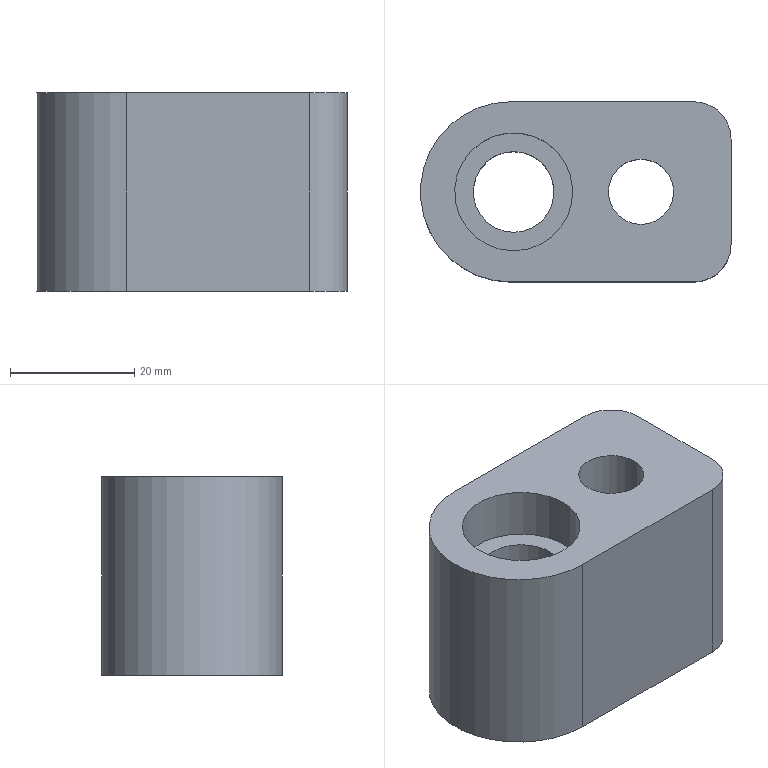Part | STEP file | lll_id118_x_t | 1 solid | 14 faces | box 50 x 29 x 32 mm | volume 32376 mm3 | plane 7 | cylinder 7 | commonest cylinder face diameters 12 x2 10.5 x1 13 x1 17 x1 19 x1 29 x1
STEP:
#1=CARTESIAN_POINT('',(792.232,22.92,60.5));
#2=VERTEX_POINT('',#1);
#3=CARTESIAN_POINT('',(792.232,29.42,60.5));
#4=DIRECTION('',(0.,0.,1.));
#5=DIRECTION('',(0.,-1.,0.));
#6=AXIS2_PLACEMENT_3D('',#3,#4,#5);
#7=CIRCLE('',#6,6.5);
#8=EDGE_CURVE('',#2,#2,#7,.T.);
#9=ORIENTED_EDGE('',*,*,#8,.T.);
#10=EDGE_LOOP('',(#9));
#11=FACE_BOUND('',#10,.T.);
#12=CARTESIAN_POINT('',(821.232,14.92,60.5));
#13=VERTEX_POINT('',#12);
#14=CARTESIAN_POINT('',(791.732,14.92,60.5));
#15=VERTEX_POINT('',#14);
#16=CARTESIAN_POINT('',(792.232,14.92,60.5));
#17=DIRECTION('',(-1.,0.,0.));
#18=VECTOR('',#17,1.);
#19=LINE('',#16,#18);
#20=EDGE_CURVE('',#13,#15,#19,.T.);
#21=ORIENTED_EDGE('',*,*,#20,.T.);
#22=CARTESIAN_POINT('',(791.732,43.92,60.5));
#23=VERTEX_POINT('',#22);
#24=CARTESIAN_POINT('',(791.732,29.42,60.5));
#25=DIRECTION('',(0.,0.,-1.));
#26=DIRECTION('',(1.,0.,0.));
#27=AXIS2_PLACEMENT_3D('',#24,#25,#26);
#28=CIRCLE('',#27,14.5);
#29=EDGE_CURVE('',#15,#23,#28,.T.);
#30=ORIENTED_EDGE('',*,*,#29,.T.);
#31=CARTESIAN_POINT('',(821.232,43.92,60.5));
#32=VERTEX_POINT('',#31);
#33=CARTESIAN_POINT('',(792.232,43.92,60.5));
#34=DIRECTION('',(1.,0.,0.));
#35=VECTOR('',#34,1.);
#36=LINE('',#33,#35);
#37=EDGE_CURVE('',#23,#32,#36,.T.);
#38=ORIENTED_EDGE('',*,*,#37,.T.);
#39=CARTESIAN_POINT('',(827.232,37.92,60.5));
#40=VERTEX_POINT('',#39);
#41=CARTESIAN_POINT('',(821.232,37.92,60.5));
#42=DIRECTION('',(0.,0.,-1.));
#43=DIRECTION('',(1.,0.,0.));
#44=AXIS2_PLACEMENT_3D('',#41,#42,#43);
#45=CIRCLE('',#44,6.);
#46=EDGE_CURVE('',#32,#40,#45,.T.);
#47=ORIENTED_EDGE('',*,*,#46,.T.);
#48=CARTESIAN_POINT('',(827.232,20.92,60.5));
#49=VERTEX_POINT('',#48);
#50=CARTESIAN_POINT('',(827.232,29.42,60.5));
#51=DIRECTION('',(0.,-1.,0.));
#52=VECTOR('',#51,1.);
#53=LINE('',#50,#52);
#54=EDGE_CURVE('',#40,#49,#53,.T.);
#55=ORIENTED_EDGE('',*,*,#54,.T.);
#56=CARTESIAN_POINT('',(821.232,20.92,60.5));
#57=DIRECTION('',(0.,0.,-1.));
#58=DIRECTION('',(0.,-1.,0.));
#59=AXIS2_PLACEMENT_3D('',#56,#57,#58);
#60=CIRCLE('',#59,6.);
#61=EDGE_CURVE('',#49,#13,#60,.T.);
#62=ORIENTED_EDGE('',*,*,#61,.T.);
#63=EDGE_LOOP('',(#21,#30,#38,#47,#55,#62));
#64=FACE_BOUND('',#63,.T.);
#65=CARTESIAN_POINT('',(812.732,20.92,60.5));
#66=VERTEX_POINT('',#65);
#67=CARTESIAN_POINT('',(812.732,29.42,60.5));
#68=DIRECTION('',(0.,0.,-1.));
#69=DIRECTION('',(0.,-1.,0.));
#70=AXIS2_PLACEMENT_3D('',#67,#68,#69);
#71=CIRCLE('',#70,8.5);
#72=EDGE_CURVE('',#66,#66,#71,.T.);
#73=ORIENTED_EDGE('',*,*,#72,.F.);
#74=EDGE_LOOP('',(#73));
#75=FACE_BOUND('',#74,.T.);
#76=CARTESIAN_POINT('',(823.457,97.56,60.5));
#77=DIRECTION('',(0.,0.,1.));
#78=DIRECTION('',(0.,1.,0.));
#79=AXIS2_PLACEMENT_3D('',#76,#77,#78);
#80=PLANE('',#79);
#81=ADVANCED_FACE('',(#11,#64,#75),#80,.F.);
#82=CARTESIAN_POINT('',(792.232,19.92,92.5));
#83=VERTEX_POINT('',#82);
#84=CARTESIAN_POINT('',(792.232,29.42,92.5));
#85=DIRECTION('',(0.,0.,1.));
#86=DIRECTION('',(0.,-1.,0.));
#87=AXIS2_PLACEMENT_3D('',#84,#85,#86);
#88=CIRCLE('',#87,9.5);
#89=EDGE_CURVE('',#83,#83,#88,.T.);
#90=ORIENTED_EDGE('',*,*,#89,.F.);
#91=EDGE_LOOP('',(#90));
#92=FACE_BOUND('',#91,.T.);
#93=CARTESIAN_POINT('',(812.732,24.17,92.5));
#94=VERTEX_POINT('',#93);
#95=CARTESIAN_POINT('',(812.732,29.42,92.5));
#96=DIRECTION('',(0.,0.,-1.));
#97=DIRECTION('',(0.,-1.,0.));
#98=AXIS2_PLACEMENT_3D('',#95,#96,#97);
#99=CIRCLE('',#98,5.25);
#100=EDGE_CURVE('',#94,#94,#99,.T.);
#101=ORIENTED_EDGE('',*,*,#100,.T.);
#102=EDGE_LOOP('',(#101));
#103=FACE_BOUND('',#102,.T.);
#104=CARTESIAN_POINT('',(791.732,43.92,92.5));
#105=VERTEX_POINT('',#104);
#106=CARTESIAN_POINT('',(791.732,14.92,92.5));
#107=VERTEX_POINT('',#106);
#108=CARTESIAN_POINT('',(791.732,29.42,92.5));
#109=DIRECTION('',(0.,0.,1.));
#110=DIRECTION('',(1.,0.,0.));
#111=AXIS2_PLACEMENT_3D('',#108,#109,#110);
#112=CIRCLE('',#111,14.5);
#113=EDGE_CURVE('',#105,#107,#112,.T.);
#114=ORIENTED_EDGE('',*,*,#113,.T.);
#115=CARTESIAN_POINT('',(821.232,14.92,92.5));
#116=VERTEX_POINT('',#115);
#117=CARTESIAN_POINT('',(792.232,14.92,92.5));
#118=DIRECTION('',(1.,0.,0.));
#119=VECTOR('',#118,1.);
#120=LINE('',#117,#119);
#121=EDGE_CURVE('',#107,#116,#120,.T.);
#122=ORIENTED_EDGE('',*,*,#121,.T.);
#123=CARTESIAN_POINT('',(827.232,20.92,92.5));
#124=VERTEX_POINT('',#123);
#125=CARTESIAN_POINT('',(821.232,20.92,92.5));
#126=DIRECTION('',(0.,0.,1.));
#127=DIRECTION('',(0.,-1.,0.));
#128=AXIS2_PLACEMENT_3D('',#125,#126,#127);
#129=CIRCLE('',#128,6.);
#130=EDGE_CURVE('',#116,#124,#129,.T.);
#131=ORIENTED_EDGE('',*,*,#130,.T.);
#132=CARTESIAN_POINT('',(827.232,37.92,92.5));
#133=VERTEX_POINT('',#132);
#134=CARTESIAN_POINT('',(827.232,29.42,92.5));
#135=DIRECTION('',(0.,1.,0.));
#136=VECTOR('',#135,1.);
#137=LINE('',#134,#136);
#138=EDGE_CURVE('',#124,#133,#137,.T.);
#139=ORIENTED_EDGE('',*,*,#138,.T.);
#140=CARTESIAN_POINT('',(821.232,43.92,92.5));
#141=VERTEX_POINT('',#140);
#142=CARTESIAN_POINT('',(821.232,37.92,92.5));
#143=DIRECTION('',(0.,0.,1.));
#144=DIRECTION('',(1.,0.,0.));
#145=AXIS2_PLACEMENT_3D('',#142,#143,#144);
#146=CIRCLE('',#145,6.);
#147=EDGE_CURVE('',#133,#141,#146,.T.);
#148=ORIENTED_EDGE('',*,*,#147,.T.);
#149=CARTESIAN_POINT('',(792.232,43.92,92.5));
#150=DIRECTION('',(-1.,0.,0.));
#151=VECTOR('',#150,1.);
#152=LINE('',#149,#151);
#153=EDGE_CURVE('',#141,#105,#152,.T.);
#154=ORIENTED_EDGE('',*,*,#153,.T.);
#155=EDGE_LOOP('',(#114,#122,#131,#139,#148,#154));
#156=FACE_BOUND('',#155,.T.);
#157=CARTESIAN_POINT('',(823.457,97.56,92.5));
#158=DIRECTION('',(0.,0.,1.));
#159=DIRECTION('',(0.,1.,0.));
#160=AXIS2_PLACEMENT_3D('',#157,#158,#159);
#161=PLANE('',#160);
#162=ADVANCED_FACE('',(#92,#103,#156),#161,.T.);
#163=ORIENTED_EDGE('',*,*,#121,.F.);
#164=CARTESIAN_POINT('',(791.732,14.92,-8.5));
#165=DIRECTION('',(0.,0.,-1.));
#166=VECTOR('',#165,1.);
#167=LINE('',#164,#166);
#168=EDGE_CURVE('',#107,#15,#167,.T.);
#169=ORIENTED_EDGE('',*,*,#168,.T.);
#170=ORIENTED_EDGE('',*,*,#20,.F.);
#171=CARTESIAN_POINT('',(821.232,14.92,-8.5));
#172=DIRECTION('',(0.,0.,1.));
#173=VECTOR('',#172,1.);
#174=LINE('',#171,#173);
#175=EDGE_CURVE('',#13,#116,#174,.T.);
#176=ORIENTED_EDGE('',*,*,#175,.T.);
#177=EDGE_LOOP('',(#163,#169,#170,#176));
#178=FACE_OUTER_BOUND('',#177,.T.);
#179=CARTESIAN_POINT('',(792.232,14.92,-8.5));
#180=DIRECTION('',(0.,-1.,0.));
#181=DIRECTION('',(0.,0.,1.));
#182=AXIS2_PLACEMENT_3D('',#179,#180,#181);
#183=PLANE('',#182);
#184=ADVANCED_FACE('',(#178),#183,.T.);
#185=ORIENTED_EDGE('',*,*,#54,.F.);
#186=CARTESIAN_POINT('',(827.232,37.92,-8.5));
#187=DIRECTION('',(0.,0.,1.));
#188=VECTOR('',#187,1.);
#189=LINE('',#186,#188);
#190=EDGE_CURVE('',#40,#133,#189,.T.);
#191=ORIENTED_EDGE('',*,*,#190,.T.);
#192=ORIENTED_EDGE('',*,*,#138,.F.);
#193=CARTESIAN_POINT('',(827.232,20.92,-8.5));
#194=DIRECTION('',(0.,0.,-1.));
#195=VECTOR('',#194,1.);
#196=LINE('',#193,#195);
#197=EDGE_CURVE('',#124,#49,#196,.T.);
#198=ORIENTED_EDGE('',*,*,#197,.T.);
#199=EDGE_LOOP('',(#185,#191,#192,#198));
#200=FACE_OUTER_BOUND('',#199,.T.);
#201=CARTESIAN_POINT('',(827.232,29.42,-8.5));
#202=DIRECTION('',(1.,0.,0.));
#203=DIRECTION('',(0.,0.,1.));
#204=AXIS2_PLACEMENT_3D('',#201,#202,#203);
#205=PLANE('',#204);
#206=ADVANCED_FACE('',(#200),#205,.T.);
#207=ORIENTED_EDGE('',*,*,#37,.F.);
#208=CARTESIAN_POINT('',(791.732,43.92,-8.5));
#209=DIRECTION('',(0.,0.,1.));
#210=VECTOR('',#209,1.);
#211=LINE('',#208,#210);
#212=EDGE_CURVE('',#23,#105,#211,.T.);
#213=ORIENTED_EDGE('',*,*,#212,.T.);
#214=ORIENTED_EDGE('',*,*,#153,.F.);
#215=CARTESIAN_POINT('',(821.232,43.92,-8.5));
#216=DIRECTION('',(0.,0.,-1.));
#217=VECTOR('',#216,1.);
#218=LINE('',#215,#217);
#219=EDGE_CURVE('',#141,#32,#218,.T.);
#220=ORIENTED_EDGE('',*,*,#219,.T.);
#221=EDGE_LOOP('',(#207,#213,#214,#220));
#222=FACE_OUTER_BOUND('',#221,.T.);
#223=CARTESIAN_POINT('',(792.232,43.92,-8.5));
#224=DIRECTION('',(0.,1.,0.));
#225=DIRECTION('',(0.,0.,-1.));
#226=AXIS2_PLACEMENT_3D('',#223,#224,#225);
#227=PLANE('',#226);
#228=ADVANCED_FACE('',(#222),#227,.T.);
#229=ORIENTED_EDGE('',*,*,#100,.F.);
#230=EDGE_LOOP('',(#229));
#231=FACE_BOUND('',#230,.T.);
#232=CARTESIAN_POINT('',(812.732,24.17,77.5));
#233=VERTEX_POINT('',#232);
#234=CARTESIAN_POINT('',(812.732,29.42,77.5));
#235=DIRECTION('',(0.,0.,1.));
#236=DIRECTION('',(0.,-1.,0.));
#237=AXIS2_PLACEMENT_3D('',#234,#235,#236);
#238=CIRCLE('',#237,5.25);
#239=EDGE_CURVE('',#233,#233,#238,.T.);
#240=ORIENTED_EDGE('',*,*,#239,.F.);
#241=EDGE_LOOP('',(#240));
#242=FACE_BOUND('',#241,.T.);
#243=CARTESIAN_POINT('',(812.732,29.42,160.5));
#244=DIRECTION('',(0.,0.,1.));
#245=DIRECTION('',(0.,1.,0.));
#246=AXIS2_PLACEMENT_3D('',#243,#244,#245);
#247=CYLINDRICAL_SURFACE('',#246,5.25);
#248=ADVANCED_FACE('',(#231,#242),#247,.F.);
#249=ORIENTED_EDGE('',*,*,#239,.T.);
#250=EDGE_LOOP('',(#249));
#251=FACE_BOUND('',#250,.T.);
#252=CARTESIAN_POINT('',(812.732,20.92,77.5));
#253=VERTEX_POINT('',#252);
#254=CARTESIAN_POINT('',(812.732,29.42,77.5));
#255=DIRECTION('',(0.,0.,1.));
#256=DIRECTION('',(0.,-1.,0.));
#257=AXIS2_PLACEMENT_3D('',#254,#255,#256);
#258=CIRCLE('',#257,8.5);
#259=EDGE_CURVE('',#253,#253,#258,.T.);
#260=ORIENTED_EDGE('',*,*,#259,.F.);
#261=EDGE_LOOP('',(#260));
#262=FACE_BOUND('',#261,.T.);
#263=CARTESIAN_POINT('',(812.732,29.42,77.5));
#264=DIRECTION('',(0.,0.,1.));
#265=DIRECTION('',(0.,1.,0.));
#266=AXIS2_PLACEMENT_3D('',#263,#264,#265);
#267=PLANE('',#266);
#268=ADVANCED_FACE('',(#251,#262),#267,.F.);
#269=ORIENTED_EDGE('',*,*,#259,.T.);
#270=EDGE_LOOP('',(#269));
#271=FACE_BOUND('',#270,.T.);
#272=ORIENTED_EDGE('',*,*,#72,.T.);
#273=EDGE_LOOP('',(#272));
#274=FACE_BOUND('',#273,.T.);
#275=CARTESIAN_POINT('',(812.732,29.42,60.5));
#276=DIRECTION('',(0.,0.,1.));
#277=DIRECTION('',(0.,1.,0.));
#278=AXIS2_PLACEMENT_3D('',#275,#276,#277);
#279=CYLINDRICAL_SURFACE('',#278,8.5);
#280=ADVANCED_FACE('',(#271,#274),#279,.F.);
#281=CARTESIAN_POINT('',(792.232,22.92,84.3));
#282=VERTEX_POINT('',#281);
#283=CARTESIAN_POINT('',(792.232,29.42,84.3));
#284=DIRECTION('',(0.,0.,1.));
#285=DIRECTION('',(0.,-1.,0.));
#286=AXIS2_PLACEMENT_3D('',#283,#284,#285);
#287=CIRCLE('',#286,6.5);
#288=EDGE_CURVE('',#282,#282,#287,.T.);
#289=ORIENTED_EDGE('',*,*,#288,.F.);
#290=EDGE_LOOP('',(#289));
#291=FACE_BOUND('',#290,.T.);
#292=CARTESIAN_POINT('',(792.232,19.92,84.3));
#293=VERTEX_POINT('',#292);
#294=CARTESIAN_POINT('',(792.232,29.42,84.3));
#295=DIRECTION('',(0.,0.,-1.));
#296=DIRECTION('',(0.,-1.,0.));
#297=AXIS2_PLACEMENT_3D('',#294,#295,#296);
#298=CIRCLE('',#297,9.5);
#299=EDGE_CURVE('',#293,#293,#298,.T.);
#300=ORIENTED_EDGE('',*,*,#299,.F.);
#301=EDGE_LOOP('',(#300));
#302=FACE_BOUND('',#301,.T.);
#303=CARTESIAN_POINT('',(792.232,29.42,84.3));
#304=DIRECTION('',(0.,0.,1.));
#305=DIRECTION('',(0.,1.,0.));
#306=AXIS2_PLACEMENT_3D('',#303,#304,#305);
#307=PLANE('',#306);
#308=ADVANCED_FACE('',(#291,#302),#307,.T.);
#309=ORIENTED_EDGE('',*,*,#288,.T.);
#310=EDGE_LOOP('',(#309));
#311=FACE_BOUND('',#310,.T.);
#312=ORIENTED_EDGE('',*,*,#8,.F.);
#313=EDGE_LOOP('',(#312));
#314=FACE_BOUND('',#313,.T.);
#315=CARTESIAN_POINT('',(792.232,29.42,124.8));
#316=DIRECTION('',(0.,0.,-1.));
#317=DIRECTION('',(0.,-1.,0.));
#318=AXIS2_PLACEMENT_3D('',#315,#316,#317);
#319=CYLINDRICAL_SURFACE('',#318,6.5);
#320=ADVANCED_FACE('',(#311,#314),#319,.F.);
#321=ORIENTED_EDGE('',*,*,#299,.T.);
#322=EDGE_LOOP('',(#321));
#323=FACE_BOUND('',#322,.T.);
#324=ORIENTED_EDGE('',*,*,#89,.T.);
#325=EDGE_LOOP('',(#324));
#326=FACE_BOUND('',#325,.T.);
#327=CARTESIAN_POINT('',(792.232,29.42,-7.5));
#328=DIRECTION('',(0.,0.,1.));
#329=DIRECTION('',(0.,1.,0.));
#330=AXIS2_PLACEMENT_3D('',#327,#328,#329);
#331=CYLINDRICAL_SURFACE('',#330,9.5);
#332=ADVANCED_FACE('',(#323,#326),#331,.F.);
#333=ORIENTED_EDGE('',*,*,#130,.F.);
#334=ORIENTED_EDGE('',*,*,#175,.F.);
#335=ORIENTED_EDGE('',*,*,#61,.F.);
#336=ORIENTED_EDGE('',*,*,#197,.F.);
#337=EDGE_LOOP('',(#333,#334,#335,#336));
#338=FACE_OUTER_BOUND('',#337,.T.);
#339=CARTESIAN_POINT('',(821.232,20.92,-8.5));
#340=DIRECTION('',(0.,0.,-1.));
#341=DIRECTION('',(0.,1.,0.));
#342=AXIS2_PLACEMENT_3D('',#339,#340,#341);
#343=CYLINDRICAL_SURFACE('',#342,6.);
#344=ADVANCED_FACE('',(#338),#343,.T.);
#345=ORIENTED_EDGE('',*,*,#147,.F.);
#346=ORIENTED_EDGE('',*,*,#190,.F.);
#347=ORIENTED_EDGE('',*,*,#46,.F.);
#348=ORIENTED_EDGE('',*,*,#219,.F.);
#349=EDGE_LOOP('',(#345,#346,#347,#348));
#350=FACE_OUTER_BOUND('',#349,.T.);
#351=CARTESIAN_POINT('',(821.232,37.92,-8.5));
#352=DIRECTION('',(0.,0.,-1.));
#353=DIRECTION('',(-1.,0.,0.));
#354=AXIS2_PLACEMENT_3D('',#351,#352,#353);
#355=CYLINDRICAL_SURFACE('',#354,6.);
#356=ADVANCED_FACE('',(#350),#355,.T.);
#357=ORIENTED_EDGE('',*,*,#29,.F.);
#358=ORIENTED_EDGE('',*,*,#168,.F.);
#359=ORIENTED_EDGE('',*,*,#113,.F.);
#360=ORIENTED_EDGE('',*,*,#212,.F.);
#361=EDGE_LOOP('',(#357,#358,#359,#360));
#362=FACE_OUTER_BOUND('',#361,.T.);
#363=CARTESIAN_POINT('',(791.732,29.42,-8.5));
#364=DIRECTION('',(0.,0.,-1.));
#365=DIRECTION('',(-1.,0.,0.));
#366=AXIS2_PLACEMENT_3D('',#363,#364,#365);
#367=CYLINDRICAL_SURFACE('',#366,14.5);
#368=ADVANCED_FACE('',(#362),#367,.T.);
#369=CLOSED_SHELL('',(#81,#162,#184,#206,#228,#248,#268,#280,#308,#320,#332,#344,#356,#368));
#370=MANIFOLD_SOLID_BREP('',#369);
#371=(LENGTH_UNIT()NAMED_UNIT(*)SI_UNIT(.MILLI.,.METRE.));
#372=UNCERTAINTY_MEASURE_WITH_UNIT(LENGTH_MEASURE(0.00002),#371,'','');
#373=(NAMED_UNIT(*)PLANE_ANGLE_UNIT()SI_UNIT($,.RADIAN.));
#374=PLANE_ANGLE_MEASURE_WITH_UNIT(PLANE_ANGLE_MEASURE(0.01745),#373);
#375=DIMENSIONAL_EXPONENTS(0.,0.,0.,0.,0.,0.,0.);
#376=(CONVERSION_BASED_UNIT('DEGREE',#374)NAMED_UNIT(#375)PLANE_ANGLE_UNIT());
#377=(NAMED_UNIT(*)SI_UNIT($,.STERADIAN.)SOLID_ANGLE_UNIT());
#378=(GEOMETRIC_REPRESENTATION_CONTEXT(3)GLOBAL_UNCERTAINTY_ASSIGNED_CONTEXT((#372))GLOBAL_UNIT_ASSIGNED_CONTEXT((#371,#376,#377))REPRESENTATION_CONTEXT('',''));
#379=ADVANCED_BREP_SHAPE_REPRESENTATION('',(#370),#378);